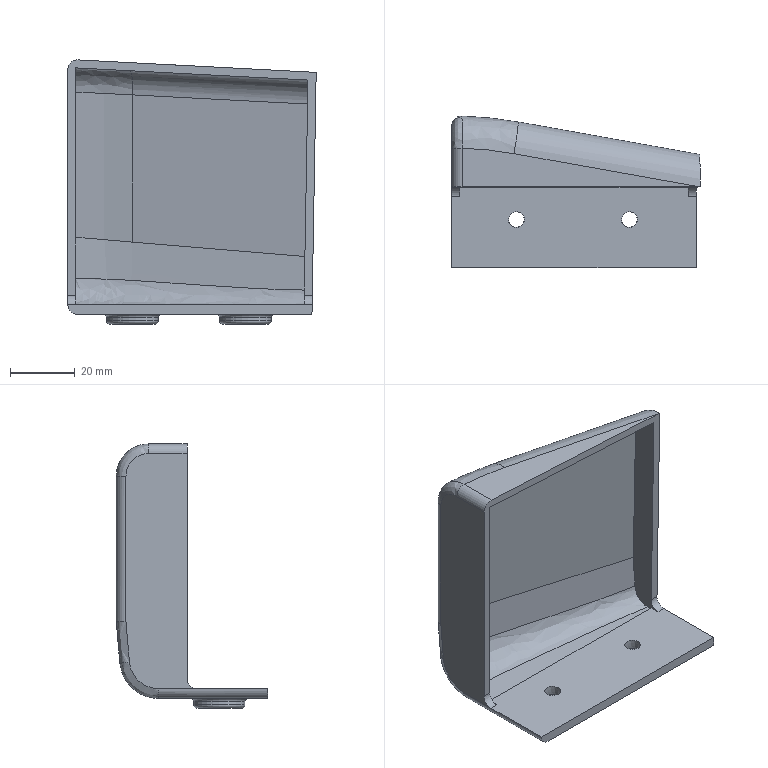Part | STEP file | HGR | 1 solid | 48 faces | box 76.93 x 46.944 x 81.839 mm | volume 29457 mm3 | plane 18 | cylinder 13 | spline 9 | torus 6 | cone 2 | commonest cylinder face diameters 6 x5 10 x2 16 x2 15 x1 20 x1 235 x1